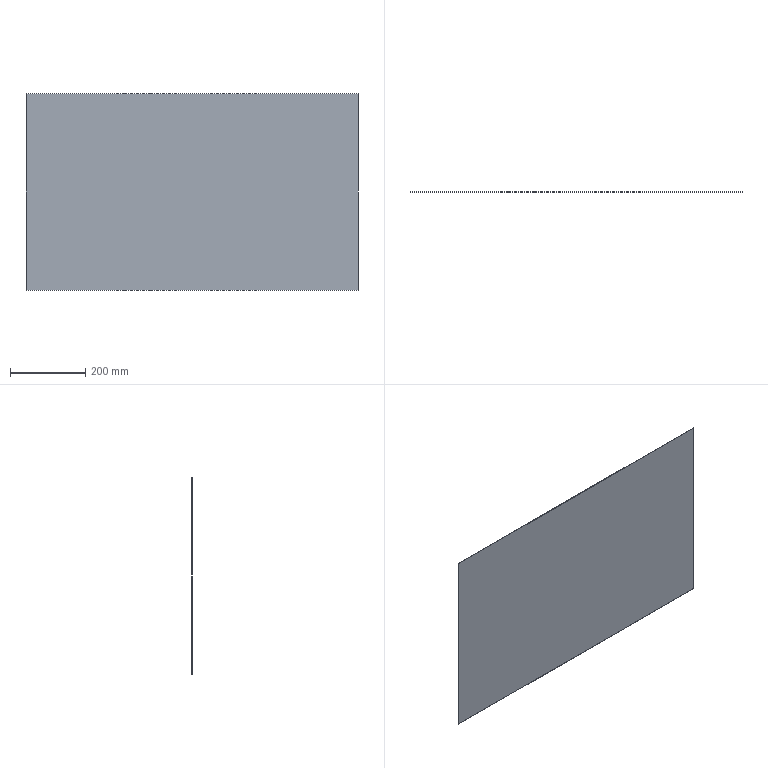Part | STEP file | Guide wheel mechanism revised.sldasm-Part-158 | 1 solid | 6 faces | box 882.42 x 1.2 x 522.42 mm | volume 553193 mm3 | plane 6
STEP:
#1=CARTESIAN_POINT('',(-441.21,1970.01,-261.21));
#2=VERTEX_POINT('',#1);
#3=CARTESIAN_POINT('',(-441.21,1970.01,261.21));
#4=VERTEX_POINT('',#3);
#5=CARTESIAN_POINT('',(-441.21,1970.01,261.21));
#6=DIRECTION('',(0.,0.,1.));
#7=VECTOR('',#6,1000.);
#8=LINE('',#5,#7);
#9=EDGE_CURVE('',#2,#4,#8,.T.);
#10=ORIENTED_EDGE('',*,*,#9,.T.);
#11=CARTESIAN_POINT('',(-441.21,1971.21,261.21));
#12=VERTEX_POINT('',#11);
#13=CARTESIAN_POINT('',(-441.21,1971.21,261.21));
#14=DIRECTION('',(0.,-1.,0.));
#15=VECTOR('',#14,1000.);
#16=LINE('',#13,#15);
#17=EDGE_CURVE('',#12,#4,#16,.T.);
#18=ORIENTED_EDGE('',*,*,#17,.F.);
#19=CARTESIAN_POINT('',(-441.21,1971.21,-261.21));
#20=VERTEX_POINT('',#19);
#21=CARTESIAN_POINT('',(-441.21,1971.21,261.21));
#22=DIRECTION('',(0.,0.,1.));
#23=VECTOR('',#22,1000.);
#24=LINE('',#21,#23);
#25=EDGE_CURVE('',#20,#12,#24,.T.);
#26=ORIENTED_EDGE('',*,*,#25,.F.);
#27=CARTESIAN_POINT('',(-441.21,1971.21,-261.21));
#28=DIRECTION('',(0.,-1.,0.));
#29=VECTOR('',#28,1000.);
#30=LINE('',#27,#29);
#31=EDGE_CURVE('',#20,#2,#30,.T.);
#32=ORIENTED_EDGE('',*,*,#31,.T.);
#33=EDGE_LOOP('',(#10,#18,#26,#32));
#34=FACE_OUTER_BOUND('',#33,.T.);
#35=CARTESIAN_POINT('',(-441.21,1971.21,261.21));
#36=DIRECTION('',(1.,0.,0.));
#37=DIRECTION('',(0.,0.,-1.));
#38=AXIS2_PLACEMENT_3D('',#35,#36,#37);
#39=PLANE('',#38);
#40=ADVANCED_FACE('',(#34),#39,.F.);
#41=CARTESIAN_POINT('',(441.21,1970.01,261.21));
#42=VERTEX_POINT('',#41);
#43=CARTESIAN_POINT('',(441.21,1970.01,261.21));
#44=DIRECTION('',(1.,0.,0.));
#45=VECTOR('',#44,1000.);
#46=LINE('',#43,#45);
#47=EDGE_CURVE('',#4,#42,#46,.T.);
#48=ORIENTED_EDGE('',*,*,#47,.T.);
#49=CARTESIAN_POINT('',(441.21,1971.21,261.21));
#50=VERTEX_POINT('',#49);
#51=CARTESIAN_POINT('',(441.21,1971.21,261.21));
#52=DIRECTION('',(0.,-1.,0.));
#53=VECTOR('',#52,1000.);
#54=LINE('',#51,#53);
#55=EDGE_CURVE('',#50,#42,#54,.T.);
#56=ORIENTED_EDGE('',*,*,#55,.F.);
#57=CARTESIAN_POINT('',(441.21,1971.21,261.21));
#58=DIRECTION('',(1.,0.,0.));
#59=VECTOR('',#58,1000.);
#60=LINE('',#57,#59);
#61=EDGE_CURVE('',#12,#50,#60,.T.);
#62=ORIENTED_EDGE('',*,*,#61,.F.);
#63=ORIENTED_EDGE('',*,*,#17,.T.);
#64=EDGE_LOOP('',(#48,#56,#62,#63));
#65=FACE_OUTER_BOUND('',#64,.T.);
#66=CARTESIAN_POINT('',(441.21,1971.21,261.21));
#67=DIRECTION('',(0.,0.,-1.));
#68=DIRECTION('',(-1.,0.,0.));
#69=AXIS2_PLACEMENT_3D('',#66,#67,#68);
#70=PLANE('',#69);
#71=ADVANCED_FACE('',(#65),#70,.F.);
#72=CARTESIAN_POINT('',(441.21,1970.01,-261.21));
#73=VERTEX_POINT('',#72);
#74=CARTESIAN_POINT('',(441.21,1970.01,261.21));
#75=DIRECTION('',(0.,0.,-1.));
#76=VECTOR('',#75,1000.);
#77=LINE('',#74,#76);
#78=EDGE_CURVE('',#42,#73,#77,.T.);
#79=ORIENTED_EDGE('',*,*,#78,.T.);
#80=CARTESIAN_POINT('',(441.21,1971.21,-261.21));
#81=VERTEX_POINT('',#80);
#82=CARTESIAN_POINT('',(441.21,1971.21,-261.21));
#83=DIRECTION('',(0.,-1.,0.));
#84=VECTOR('',#83,1000.);
#85=LINE('',#82,#84);
#86=EDGE_CURVE('',#81,#73,#85,.T.);
#87=ORIENTED_EDGE('',*,*,#86,.F.);
#88=CARTESIAN_POINT('',(441.21,1971.21,261.21));
#89=DIRECTION('',(0.,0.,-1.));
#90=VECTOR('',#89,1000.);
#91=LINE('',#88,#90);
#92=EDGE_CURVE('',#50,#81,#91,.T.);
#93=ORIENTED_EDGE('',*,*,#92,.F.);
#94=ORIENTED_EDGE('',*,*,#55,.T.);
#95=EDGE_LOOP('',(#79,#87,#93,#94));
#96=FACE_OUTER_BOUND('',#95,.T.);
#97=CARTESIAN_POINT('',(441.21,1971.21,261.21));
#98=DIRECTION('',(-1.,0.,0.));
#99=DIRECTION('',(0.,0.,1.));
#100=AXIS2_PLACEMENT_3D('',#97,#98,#99);
#101=PLANE('',#100);
#102=ADVANCED_FACE('',(#96),#101,.F.);
#103=CARTESIAN_POINT('',(441.21,1970.01,-261.21));
#104=DIRECTION('',(-1.,0.,0.));
#105=VECTOR('',#104,1000.);
#106=LINE('',#103,#105);
#107=EDGE_CURVE('',#73,#2,#106,.T.);
#108=ORIENTED_EDGE('',*,*,#107,.T.);
#109=ORIENTED_EDGE('',*,*,#31,.F.);
#110=CARTESIAN_POINT('',(441.21,1971.21,-261.21));
#111=DIRECTION('',(-1.,0.,0.));
#112=VECTOR('',#111,1000.);
#113=LINE('',#110,#112);
#114=EDGE_CURVE('',#81,#20,#113,.T.);
#115=ORIENTED_EDGE('',*,*,#114,.F.);
#116=ORIENTED_EDGE('',*,*,#86,.T.);
#117=EDGE_LOOP('',(#108,#109,#115,#116));
#118=FACE_OUTER_BOUND('',#117,.T.);
#119=CARTESIAN_POINT('',(441.21,1971.21,-261.21));
#120=DIRECTION('',(0.,0.,1.));
#121=DIRECTION('',(1.,0.,0.));
#122=AXIS2_PLACEMENT_3D('',#119,#120,#121);
#123=PLANE('',#122);
#124=ADVANCED_FACE('',(#118),#123,.F.);
#125=ORIENTED_EDGE('',*,*,#25,.T.);
#126=ORIENTED_EDGE('',*,*,#61,.T.);
#127=ORIENTED_EDGE('',*,*,#92,.T.);
#128=ORIENTED_EDGE('',*,*,#114,.T.);
#129=EDGE_LOOP('',(#125,#126,#127,#128));
#130=FACE_OUTER_BOUND('',#129,.T.);
#131=CARTESIAN_POINT('',(0.,1971.21,0.));
#132=DIRECTION('',(0.,1.,0.));
#133=DIRECTION('',(0.,0.,1.));
#134=AXIS2_PLACEMENT_3D('',#131,#132,#133);
#135=PLANE('',#134);
#136=ADVANCED_FACE('',(#130),#135,.T.);
#137=ORIENTED_EDGE('',*,*,#9,.F.);
#138=ORIENTED_EDGE('',*,*,#107,.F.);
#139=ORIENTED_EDGE('',*,*,#78,.F.);
#140=ORIENTED_EDGE('',*,*,#47,.F.);
#141=EDGE_LOOP('',(#137,#138,#139,#140));
#142=FACE_OUTER_BOUND('',#141,.T.);
#143=CARTESIAN_POINT('',(0.,1970.01,0.));
#144=DIRECTION('',(0.,1.,0.));
#145=DIRECTION('',(0.,0.,1.));
#146=AXIS2_PLACEMENT_3D('',#143,#144,#145);
#147=PLANE('',#146);
#148=ADVANCED_FACE('',(#142),#147,.F.);
#149=CLOSED_SHELL('',(#40,#71,#102,#124,#136,#148));
#150=MANIFOLD_SOLID_BREP('',#149);
#151=CARTESIAN_POINT('',(0.,0.,0.));
#152=DIRECTION('',(0.,0.,1.));
#153=DIRECTION('',(1.,0.,0.));
#154=AXIS2_PLACEMENT_3D('',#151,#152,#153);
#155=(LENGTH_UNIT()NAMED_UNIT(*)SI_UNIT(.MILLI.,.METRE.));
#156=UNCERTAINTY_MEASURE_WITH_UNIT(LENGTH_MEASURE(0.00001),#155,'','');
#157=(NAMED_UNIT(*)PLANE_ANGLE_UNIT()SI_UNIT($,.RADIAN.));
#158=(NAMED_UNIT(*)SI_UNIT($,.STERADIAN.)SOLID_ANGLE_UNIT());
#159=(GEOMETRIC_REPRESENTATION_CONTEXT(3)GLOBAL_UNCERTAINTY_ASSIGNED_CONTEXT((#156))GLOBAL_UNIT_ASSIGNED_CONTEXT((#155,#157,#158))REPRESENTATION_CONTEXT('',''));
#160=ADVANCED_BREP_SHAPE_REPRESENTATION('',(#150,#154),#159);